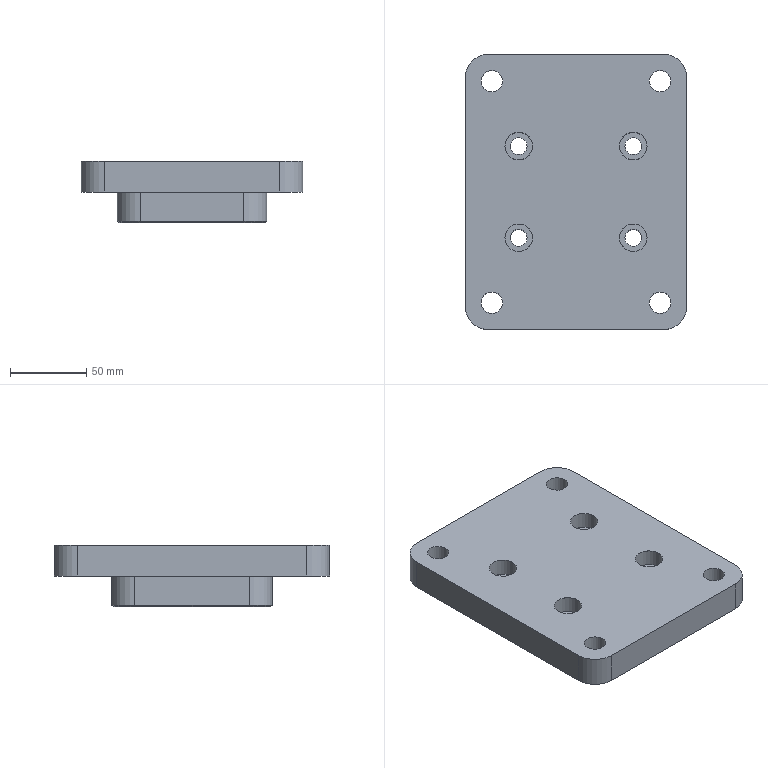NC program | NX | posted with a generic post | part box 145 x 180 x 40 mm
Lines 40 to 1301 of 5818:
(ZLEVEL_PROFILE_1_COPY , TOOL : D10)
N72 T10 M6
N74 G54
N76 G17 G0 G90 X71.61 Y79.6 S3200 M3
N78 G43 Z30. H10
N80 Z1.78
N82 G94 G1 Z-0.22 F2200.
N84 X72.478 Y78.099
N86 G3 X73.345 Y77.599 R1.
N88 G1 X74.677 Y77.6
N90 X75.
N92 G2 X95.1 Y57.5 R20.1
N94 G1 Y57.177
N96 Y55.845
N98 G3 X95.6 Y54.979 R1.
N100 G1 X97.1 Y54.112
N102 Z1.78
N104 G0 Z30.
N106 Z1.56
N108 G1 Z-0.44
N110 X95.6 Y54.979
N112 G2 X95.1 Y55.845 R1.
N114 G1 Y57.177
N116 Y57.5
N118 G3 X75. Y77.6 R20.1
N120 G1 X74.677
N122 X73.345 Y77.599
N124 G2 X72.478 Y78.099 R1.
N126 G1 X71.61 Y79.6
N128 Z1.56
N130 G0 Z30.
N132 Z1.341
N134 G1 Z-0.659
N136 X72.478 Y78.099
N138 G3 X73.345 Y77.599 R1.
N140 G1 X74.677 Y77.6
N142 X75.
N144 G2 X95.1 Y57.5 R20.1
N146 G1 Y57.177
N148 Y55.845
N150 G3 X95.6 Y54.979 R1.
N152 G1 X97.1 Y54.112
N154 Z1.341
N156 G0 Z30.
N158 Z1.121
N160 G1 Z-0.879
N162 X95.6 Y54.979
N164 G2 X95.1 Y55.845 R1.
N166 G1 Y57.177
N168 Y57.5
N170 G3 X75. Y77.6 R20.1
N172 G1 X74.677
N174 X73.345 Y77.599
N176 G2 X72.478 Y78.099 R1.
N178 G1 X71.61 Y79.6
N180 Z1.121
N182 G0 Z30.
N184 Z0.901
N186 G1 Z-1.099
N188 X72.478 Y78.099
N190 G3 X73.345 Y77.599 R1.
N192 G1 X74.677 Y77.6
N194 X75.
N196 G2 X95.1 Y57.5 R20.1
N198 G1 Y57.177
N200 Y55.845
N202 G3 X95.6 Y54.979 R1.
N204 G1 X97.1 Y54.112
N206 Z0.901
N208 G0 Z30.
N210 Z0.681
N212 G1 Z-1.319
N214 X95.6 Y54.979
N216 G2 X95.1 Y55.845 R1.
N218 G1 Y57.177
N220 Y57.5
N222 G3 X75. Y77.6 R20.1
N224 G1 X74.677
N226 X73.345 Y77.599
N228 G2 X72.478 Y78.099 R1.
N230 G1 X71.61 Y79.6
N232 Z0.681
N234 G0 Z30.
N236 Z0.462
N238 G1 Z-1.538
N240 X72.478 Y78.099
N242 G3 X73.345 Y77.599 R1.
N244 G1 X74.677 Y77.6
N246 X75.
N248 G2 X95.1 Y57.5 R20.1
N250 G1 Y57.177
N252 Y55.845
N254 G3 X95.6 Y54.979 R1.
N256 G1 X97.1 Y54.112
N258 Z0.462
N260 G0 Z30.
N262 Z0.242
N264 G1 Z-1.758
N266 X95.6 Y54.979
N268 G2 X95.1 Y55.845 R1.
N270 G1 Y57.177
N272 Y57.5
N274 G3 X75. Y77.6 R20.1
N276 G1 X74.677
N278 X73.345 Y77.599
N280 G2 X72.478 Y78.099 R1.
N282 G1 X71.61 Y79.6
N284 Z0.242
N286 G0 Z30.
N288 Z0.022
N290 G1 Z-1.978
N292 X72.478 Y78.099
N294 G3 X73.345 Y77.599 R1.
N296 G1 X74.677 Y77.6
N298 X75.
N300 G2 X95.1 Y57.5 R20.1
N302 G1 Y57.177
N304 Y55.845
N306 G3 X95.6 Y54.979 R1.
N308 G1 X97.1 Y54.112
N310 Z0.022
N312 G0 Z30.
N314 Z-0.198
N316 G1 Z-2.198
N318 X95.6 Y54.979
N320 G2 X95.1 Y55.845 R1.
N322 G1 Y57.177
N324 Y57.5
N326 G3 X75. Y77.6 R20.1
N328 G1 X74.677
N330 X73.345 Y77.599
N332 G2 X72.478 Y78.099 R1.
N334 G1 X71.61 Y79.6
N336 Z-0.198
N338 G0 Z30.
N340 Z-0.418
N342 G1 Z-2.418
N344 X72.478 Y78.099
N346 G3 X73.345 Y77.599 R1.
N348 G1 X74.677 Y77.6
N350 X75.
N352 G2 X95.1 Y57.5 R20.1
N354 G1 Y57.177
N356 Y55.845
N358 G3 X95.6 Y54.979 R1.
N360 G1 X97.1 Y54.112
N362 Z-0.418
N364 G0 Z30.
N366 Z-0.637
N368 G1 Z-2.637
N370 X95.6 Y54.979
N372 G2 X95.1 Y55.845 R1.
N374 G1 Y57.177
N376 Y57.5
N378 G3 X75. Y77.6 R20.1
N380 G1 X74.677
N382 X73.345 Y77.599
N384 G2 X72.478 Y78.099 R1.
N386 G1 X71.61 Y79.6
N388 Z-0.637
N390 G0 Z30.
N392 Z-0.857
N394 G1 Z-2.857
N396 X72.478 Y78.099
N398 G3 X73.345 Y77.599 R1.
N400 G1 X74.677 Y77.6
N402 X75.
N404 G2 X95.1 Y57.5 R20.1
N406 G1 Y57.177
N408 Y55.845
N410 G3 X95.6 Y54.979 R1.
N412 G1 X97.1 Y54.112
N414 Z-0.857
N416 G0 Z30.
N418 Z-1.077
N420 G1 Z-3.077
N422 X95.6 Y54.979
N424 G2 X95.1 Y55.845 R1.
N426 G1 Y57.177
N428 Y57.5
N430 G3 X75. Y77.6 R20.1
N432 G1 X74.677
N434 X73.345 Y77.599
N436 G2 X72.478 Y78.099 R1.
N438 G1 X71.61 Y79.6
N440 Z-1.077
N442 G0 Z30.
N444 Z-1.297
N446 G1 Z-3.297
N448 X72.478 Y78.099
N450 G3 X73.345 Y77.599 R1.
N452 G1 X74.677 Y77.6
N454 X75.
N456 G2 X95.1 Y57.5 R20.1
N458 G1 Y57.177
N460 Y55.845
N462 G3 X95.6 Y54.979 R1.
N464 G1 X97.1 Y54.112
N466 Z-1.297
N468 G0 Z30.
N470 Z-1.516
N472 G1 Z-3.516
N474 X95.6 Y54.979
N476 G2 X95.1 Y55.845 R1.
N478 G1 Y57.177
N480 Y57.5
N482 G3 X75. Y77.6 R20.1
N484 G1 X74.677
N486 X73.345 Y77.599
N488 G2 X72.478 Y78.099 R1.
N490 G1 X71.61 Y79.6
N492 Z-1.516
N494 G0 Z30.
N496 Z-1.736
N498 G1 Z-3.736
N500 X72.478 Y78.099
N502 G3 X73.345 Y77.599 R1.
N504 G1 X74.677 Y77.6
N506 X75.
N508 G2 X95.1 Y57.5 R20.1
N510 G1 Y57.177
N512 Y55.845
N514 G3 X95.6 Y54.979 R1.
N516 G1 X97.1 Y54.112
N518 Z-1.736
N520 G0 Z30.
N522 Z-1.956
N524 G1 Z-3.956
N526 X95.6 Y54.979
N528 G2 X95.1 Y55.845 R1.
N530 G1 Y57.177
N532 Y57.5
N534 G3 X75. Y77.6 R20.1
N536 G1 X74.677
N538 X73.345 Y77.599
N540 G2 X72.478 Y78.099 R1.
N542 G1 X71.61 Y79.6
N544 Z-1.956
N546 G0 Z30.
N548 Z-2.176
N550 G1 Z-4.176
N552 X72.478 Y78.099
N554 G3 X73.345 Y77.599 R1.
N556 G1 X74.677 Y77.6
N558 X75.
N560 G2 X95.1 Y57.5 R20.1
N562 G1 Y57.177
N564 Y55.845
N566 G3 X95.6 Y54.979 R1.
N568 G1 X97.1 Y54.112
N570 Z-2.176
N572 G0 Z30.
N574 Z-2.396
N576 G1 Z-4.396
N578 X95.6 Y54.979
N580 G2 X95.1 Y55.845 R1.
N582 G1 Y57.177
N584 Y57.5
N586 G3 X75. Y77.6 R20.1
N588 G1 X74.677
N590 X73.345 Y77.599
N592 G2 X72.478 Y78.099 R1.
N594 G1 X71.61 Y79.6
N596 Z-2.396
N598 G0 Z30.
N600 Z-2.615
N602 G1 Z-4.615
N604 X72.478 Y78.099
N606 G3 X73.345 Y77.599 R1.
N608 G1 X74.677 Y77.6
N610 X75.
N612 G2 X95.1 Y57.5 R20.1
N614 G1 Y57.177
N616 Y55.845
N618 G3 X95.6 Y54.979 R1.
N620 G1 X97.1 Y54.112
N622 Z-2.615
N624 G0 Z30.
N626 Z-2.835
N628 G1 Z-4.835
N630 X95.6 Y54.979
N632 G2 X95.1 Y55.845 R1.
N634 G1 Y57.177
N636 Y57.5
N638 G3 X75. Y77.6 R20.1
N640 G1 X74.677
N642 X73.345 Y77.599
N644 G2 X72.478 Y78.099 R1.
N646 G1 X71.61 Y79.6
N648 Z-2.835
N650 G0 Z30.
N652 Z-3.055
N654 G1 Z-5.055
N656 X72.478 Y78.099
N658 G3 X73.345 Y77.599 R1.
N660 G1 X74.677 Y77.6
N662 X75.
N664 G2 X95.1 Y57.5 R20.1
N666 G1 Y57.177
N668 Y55.845
N670 G3 X95.6 Y54.979 R1.
N672 G1 X97.1 Y54.112
N674 Z-3.055
N676 G0 Z30.
N678 Z-3.275
N680 G1 Z-5.275
N682 X95.6 Y54.979
N684 G2 X95.1 Y55.845 R1.
N686 G1 Y57.177
N688 Y57.5
N690 G3 X75. Y77.6 R20.1
N692 G1 X74.677
N694 X73.345 Y77.599
N696 G2 X72.478 Y78.099 R1.
N698 G1 X71.61 Y79.6
N700 Z-3.275
N702 G0 Z30.
N704 Z-3.495
N706 G1 Z-5.495
N708 X72.478 Y78.099
N710 G3 X73.345 Y77.599 R1.
N712 G1 X74.677 Y77.6
N714 X75.
N716 G2 X95.1 Y57.5 R20.1
N718 G1 Y57.177
N720 Y55.845
N722 G3 X95.6 Y54.979 R1.
N724 G1 X97.1 Y54.112
N726 Z-3.495
N728 G0 Z30.
N730 Z-3.714
N732 G1 Z-5.714
N734 X95.6 Y54.979
N736 G2 X95.1 Y55.845 R1.
N738 G1 Y57.177
N740 Y57.5
N742 G3 X75. Y77.6 R20.1
N744 G1 X74.677
N746 X73.345 Y77.599
N748 G2 X72.478 Y78.099 R1.
N750 G1 X71.61 Y79.6
N752 Z-3.714
N754 G0 Z30.
N756 Z-3.934
N758 G1 Z-5.934
N760 X72.478 Y78.099
N762 G3 X73.345 Y77.599 R1.
N764 G1 X74.677 Y77.6
N766 X75.
N768 G2 X95.1 Y57.5 R20.1
N770 G1 Y57.177
N772 Y55.845
N774 G3 X95.6 Y54.979 R1.
N776 G1 X97.1 Y54.112
N778 Z-3.934
N780 G0 Z30.
N782 Z-4.154
N784 G1 Z-6.154
N786 X95.6 Y54.979
N788 G2 X95.1 Y55.845 R1.
N790 G1 Y57.177
N792 Y57.5
N794 G3 X75. Y77.6 R20.1
N796 G1 X74.677
N798 X73.345 Y77.599
N800 G2 X72.478 Y78.099 R1.
N802 G1 X71.61 Y79.6
N804 Z-4.154
N806 G0 Z30.
N808 Z-4.374
N810 G1 Z-6.374
N812 X72.478 Y78.099
N814 G3 X73.345 Y77.599 R1.
N816 G1 X74.677 Y77.6
N818 X75.
N820 G2 X95.1 Y57.5 R20.1
N822 G1 Y57.177
N824 Y55.845
N826 G3 X95.6 Y54.979 R1.
N828 G1 X97.1 Y54.112
N830 Z-4.374
N832 G0 Z30.
N834 Z-4.593
N836 G1 Z-6.593
N838 X95.6 Y54.979
N840 G2 X95.1 Y55.845 R1.
N842 G1 Y57.177
N844 Y57.5
N846 G3 X75. Y77.6 R20.1
N848 G1 X74.677
N850 X73.345 Y77.599
N852 G2 X72.478 Y78.099 R1.
N854 G1 X71.61 Y79.6
N856 Z-4.593
N858 G0 Z30.
N860 Z-4.813
N862 G1 Z-6.813
N864 X72.478 Y78.099
N866 G3 X73.345 Y77.599 R1.
N868 G1 X74.677 Y77.6
N870 X75.
N872 G2 X95.1 Y57.5 R20.1
N874 G1 Y57.177
N876 Y55.845
N878 G3 X95.6 Y54.979 R1.
N880 G1 X97.1 Y54.112
N882 Z-4.813
N884 G0 Z30.
N886 Z-5.033
N888 G1 Z-7.033
N890 X95.6 Y54.979
N892 G2 X95.1 Y55.845 R1.
N894 G1 Y57.177
N896 Y57.5
N898 G3 X75. Y77.6 R20.1
N900 G1 X74.677
N902 X73.345 Y77.599
N904 G2 X72.478 Y78.099 R1.
N906 G1 X71.61 Y79.6
N908 Z-5.033
N910 G0 Z30.
N912 Z-5.253
N914 G1 Z-7.253
N916 X72.478 Y78.099
N918 G3 X73.345 Y77.599 R1.
N920 G1 X74.677 Y77.6
N922 X75.
N924 G2 X95.1 Y57.5 R20.1
N926 G1 Y57.177
N928 Y55.845
N930 G3 X95.6 Y54.979 R1.
N932 G1 X97.1 Y54.112
N934 Z-5.253
N936 G0 Z30.
N938 Z-5.473
N940 G1 Z-7.473
N942 X95.6 Y54.979
N944 G2 X95.1 Y55.845 R1.
N946 G1 Y57.177
N948 Y57.5
N950 G3 X75. Y77.6 R20.1
N952 G1 X74.677
N954 X73.345 Y77.599
N956 G2 X72.478 Y78.099 R1.
N958 G1 X71.61 Y79.6
N960 Z-5.473
N962 G0 Z30.
N964 Z-5.692
N966 G1 Z-7.692
N968 X72.478 Y78.099
N970 G3 X73.345 Y77.599 R1.
N972 G1 X74.677 Y77.6
N974 X75.
N976 G2 X95.1 Y57.5 R20.1
N978 G1 Y57.177
N980 Y55.845
N982 G3 X95.6 Y54.979 R1.
N984 G1 X97.1 Y54.112
N986 Z-5.692
N988 G0 Z30.
N990 Z-5.912
N992 G1 Z-7.912
N994 X95.6 Y54.979
N996 G2 X95.1 Y55.845 R1.
N998 G1 Y57.177
N1000 Y57.5
N1002 G3 X75. Y77.6 R20.1
N1004 G1 X74.677
N1006 X73.345 Y77.599
N1008 G2 X72.478 Y78.099 R1.
N1010 G1 X71.61 Y79.6
N1012 Z-5.912
N1014 G0 Z30.
N1016 Z-6.132
N1018 G1 Z-8.132
N1020 X72.478 Y78.099
N1022 G3 X73.345 Y77.599 R1.
N1024 G1 X74.677 Y77.6
N1026 X75.
N1028 G2 X95.1 Y57.5 R20.1
N1030 G1 Y57.177
N1032 Y55.845
N1034 G3 X95.6 Y54.979 R1.
N1036 G1 X97.1 Y54.112
N1038 Z-6.132
N1040 G0 Z30.
N1042 Z-6.352
N1044 G1 Z-8.352
N1046 X95.6 Y54.979
N1048 G2 X95.1 Y55.845 R1.
N1050 G1 Y57.177
N1052 Y57.5
N1054 G3 X75. Y77.6 R20.1
N1056 G1 X74.677
N1058 X73.345 Y77.599
N1060 G2 X72.478 Y78.099 R1.
N1062 G1 X71.61 Y79.6
N1064 Z-6.352
N1066 G0 Z30.
N1068 Z-6.571
N1070 G1 Z-8.571
N1072 X72.478 Y78.099
N1074 G3 X73.345 Y77.599 R1.
N1076 G1 X74.677 Y77.6
N1078 X75.
N1080 G2 X95.1 Y57.5 R20.1
N1082 G1 Y57.177
N1084 Y55.845
N1086 G3 X95.6 Y54.979 R1.
N1088 G1 X97.1 Y54.112
N1090 Z-6.571
N1092 G0 Z30.
N1094 Z-6.791
N1096 G1 Z-8.791
N1098 X95.6 Y54.979
N1100 G2 X95.1 Y55.845 R1.
N1102 G1 Y57.177
N1104 Y57.5
N1106 G3 X75. Y77.6 R20.1
N1108 G1 X74.677
N1110 X73.345 Y77.599
N1112 G2 X72.478 Y78.099 R1.
N1114 G1 X71.61 Y79.6
N1116 Z-6.791
N1118 G0 Z30.
N1120 Z-7.011
N1122 G1 Z-9.011
N1124 X72.478 Y78.099
N1126 G3 X73.345 Y77.599 R1.
N1128 G1 X74.677 Y77.6
N1130 X75.
N1132 G2 X95.1 Y57.5 R20.1
N1134 G1 Y57.177
N1136 Y55.845
N1138 G3 X95.6 Y54.979 R1.
N1140 G1 X97.1 Y54.112
N1142 Z-7.011
N1144 G0 Z30.
N1146 Z-7.231
N1148 G1 Z-9.231
N1150 X95.6 Y54.979
N1152 G2 X95.1 Y55.845 R1.
N1154 G1 Y57.177
N1156 Y57.5
N1158 G3 X75. Y77.6 R20.1
N1160 G1 X74.677
N1162 X73.345 Y77.599
N1164 G2 X72.478 Y78.099 R1.
N1166 G1 X71.61 Y79.6
N1168 Z-7.231
N1170 G0 Z30.
N1172 Z-7.451
N1174 G1 Z-9.451
N1176 X72.478 Y78.099
N1178 G3 X73.345 Y77.599 R1.
N1180 G1 X74.677 Y77.6
N1182 X75.
N1184 G2 X95.1 Y57.5 R20.1
N1186 G1 Y57.177
N1188 Y55.845
N1190 G3 X95.6 Y54.979 R1.
N1192 G1 X97.1 Y54.112
N1194 Z-7.451
N1196 G0 Z30.
N1198 Z-7.67
N1200 G1 Z-9.67
N1202 X95.6 Y54.979
N1204 G2 X95.1 Y55.845 R1.
N1206 G1 Y57.177
N1208 Y57.5
N1210 G3 X75. Y77.6 R20.1
N1212 G1 X74.677
N1214 X73.345 Y77.599
N1216 G2 X72.478 Y78.099 R1.
N1218 G1 X71.61 Y79.6
N1220 Z-7.67
N1222 G0 Z30.
N1224 Z-7.89
N1226 G1 Z-9.89
N1228 X72.478 Y78.099
N1230 G3 X73.345 Y77.599 R1.
N1232 G1 X74.677 Y77.6
N1234 X75.
N1236 G2 X95.1 Y57.5 R20.1
N1238 G1 Y57.177
N1240 Y55.845
N1242 G3 X95.6 Y54.979 R1.
N1244 G1 X97.1 Y54.112
N1246 Z-7.89
N1248 G0 Z30.
N1250 Z-8.11
N1252 G1 Z-10.11
N1254 X95.6 Y54.979
N1256 G2 X95.1 Y55.845 R1.
N1258 G1 Y57.177
N1260 Y57.5
N1262 G3 X75. Y77.6 R20.1
N1264 G1 X74.677
N1266 X73.345 Y77.599
N1268 G2 X72.478 Y78.099 R1.
N1270 G1 X71.61 Y79.6
N1272 Z-8.11
N1274 G0 Z30.
N1276 X71.611 Z-8.33
N1278 G1 Z-10.33
N1280 X72.478 Y78.099
N1282 G3 X73.345 Y77.599 R1.
N1284 G1 X74.677 Y77.6
N1286 X75.
N1288 G2 X95.1 Y57.5 R20.1
N1290 G1 Y57.177
N1292 Y55.845
N1294 G3 X95.6 Y54.979 R1.
N1296 G1 X97.1 Y54.112
N1298 Z-8.33
N1300 G0 Z30.
N1302 Z-8.549
N1304 G1 Z-10.549
N1306 X95.6 Y54.979
N1308 G2 X95.1 Y55.845 R1.
N1310 G1 Y57.177
N1312 Y57.5
N1314 G3 X75. Y77.6 R20.1
N1316 G1 X74.677
N1318 X73.345 Y77.599
N1320 G2 X72.478 Y78.099 R1.
N1322 G1 X71.611 Y79.6
N1324 Z-8.549
N1326 G0 Z30.
N1328 Z-8.769
N1330 G1 Z-10.769
N1332 X72.478 Y78.099
N1334 G3 X73.345 Y77.599 R1.
N1336 G1 X74.677 Y77.6
N1338 X75.
N1340 G2 X95.1 Y57.5 R20.1
N1342 G1 Y57.177
N1344 Y55.845
N1346 G3 X95.6 Y54.979 R1.
N1348 G1 X97.1 Y54.112
N1350 Z-8.769
N1352 G0 Z30.
N1354 Z-8.989
N1356 G1 Z-10.989
N1358 X95.6 Y54.979
N1360 G2 X95.1 Y55.845 R1.
N1362 G1 Y57.177
N1364 Y57.5
N1366 G3 X75. Y77.6 R20.1
N1368 G1 X74.677
N1370 X73.345 Y77.599
N1372 G2 X72.478 Y78.099 R1.
N1374 G1 X71.611 Y79.6
N1376 Z-8.989
N1378 G0 Z30.
N1380 Z-9.209
N1382 G1 Z-11.209
N1384 X72.478 Y78.099
N1386 G3 X73.345 Y77.599 R1.
N1388 G1 X74.677 Y77.6
N1390 X75.
N1392 G2 X95.1 Y57.5 R20.1
N1394 G1 Y57.177
N1396 Y55.845
N1398 G3 X95.6 Y54.979 R1.
N1400 G1 X97.1 Y54.112
N1402 Z-9.209
N1404 G0 Z30.
N1406 Z-9.429
N1408 G1 Z-11.429
N1410 X95.6 Y54.979
N1412 G2 X95.1 Y55.845 R1.
N1414 G1 Y57.177
N1416 Y57.5
N1418 G3 X75. Y77.6 R20.1
N1420 G1 X74.677
N1422 X73.345 Y77.599
N1424 G2 X72.478 Y78.099 R1.
N1426 G1 X71.611 Y79.6
N1428 Z-9.429
N1430 G0 Z30.
N1432 Z-9.648
N1434 G1 Z-11.648
N1436 X72.478 Y78.099
N1438 G3 X73.345 Y77.599 R1.
N1440 G1 X74.677 Y77.6
N1442 X75.
N1444 G2 X95.1 Y57.5 R20.1
N1446 G1 Y57.177
N1448 Y55.845
N1450 G3 X95.6 Y54.979 R1.
N1452 G1 X97.1 Y54.112
N1454 Z-9.648
N1456 G0 Z30.
N1458 Z-9.868
N1460 G1 Z-11.868
N1462 X95.6 Y54.979
N1464 G2 X95.1 Y55.845 R1.
N1466 G1 Y57.177
N1468 Y57.5
N1470 G3 X75. Y77.6 R20.1
N1472 G1 X74.677
N1474 X73.345 Y77.599
N1476 G2 X72.478 Y78.099 R1.
N1478 G1 X71.611 Y79.6
N1480 Z-9.868
N1482 G0 Z30.
N1484 Z-10.088
N1486 G1 Z-12.088
N1488 X72.478 Y78.099
N1490 G3 X73.345 Y77.599 R1.
N1492 G1 X74.677 Y77.6
N1494 X75.
N1496 G2 X95.1 Y57.5 R20.1
N1498 G1 Y57.177
N1500 Y55.845
N1502 G3 X95.6 Y54.979 R1.
N1504 G1 X97.1 Y54.112
N1506 Z-10.088
N1508 G0 Z30.
N1510 Z-10.308
N1512 G1 Z-12.308
N1514 X95.6 Y54.979
N1516 G2 X95.1 Y55.845 R1.
N1518 G1 Y57.177
N1520 Y57.5
N1522 G3 X75. Y77.6 R20.1
N1524 G1 X74.677
N1526 X73.345 Y77.599
N1528 G2 X72.478 Y78.099 R1.
N1530 G1 X71.611 Y79.6
N1532 Z-10.308
N1534 G0 Z30.
N1536 Z-10.527
N1538 G1 Z-12.527
N1540 X72.478 Y78.099
N1542 G3 X73.345 Y77.599 R1.
N1544 G1 X74.677 Y77.6
N1546 X75.
N1548 G2 X95.1 Y57.5 R20.1
N1550 G1 Y57.177
N1552 Y55.845
N1554 G3 X95.6 Y54.979 R1.
N1556 G1 X97.1 Y54.112
N1558 Z-10.527
N1560 G0 Z30.
N1562 Z-10.747
N1564 G1 Z-12.747
N1566 X95.6 Y54.979
N1568 G2 X95.1 Y55.845 R1.
N1570 G1 Y57.177
N1572 Y57.5
N1574 G3 X75. Y77.6 R20.1
N1576 G1 X74.677
N1578 X73.345 Y77.599
N1580 G2 X72.478 Y78.099 R1.
N1582 G1 X71.611 Y79.6
N1584 Z-10.747
N1586 G0 Z30.
N1588 Z-10.967
N1590 G1 Z-12.967
N1592 X72.478 Y78.099
N1594 G3 X73.345 Y77.599 R1.
N1596 G1 X74.677 Y77.6
N1598 X75.
N1600 G2 X95.1 Y57.5 R20.1
N1602 G1 Y57.177
N1604 Y55.845
N1606 G3 X95.6 Y54.979 R1.
N1608 G1 X97.1 Y54.112
N1610 Z-10.967
N1612 G0 Z30.
N1614 Z-11.187
N1616 G1 Z-13.187
N1618 X95.6 Y54.979
N1620 G2 X95.1 Y55.845 R1.
N1622 G1 Y57.177
N1624 Y57.5
N1626 G3 X75. Y77.6 R20.1
N1628 G1 X74.677
N1630 X73.345 Y77.599
N1632 G2 X72.478 Y78.099 R1.
N1634 G1 X71.611 Y79.6
N1636 Z-11.187
N1638 G0 Z30.
N1640 Z-11.407
N1642 G1 Z-13.407
N1644 X72.478 Y78.099
N1646 G3 X73.345 Y77.599 R1.
N1648 G1 X74.677 Y77.6
N1650 X75.
N1652 G2 X95.1 Y57.5 R20.1
N1654 G1 Y57.177
N1656 Y55.845
N1658 G3 X95.6 Y54.979 R1.
N1660 G1 X97.1 Y54.112
N1662 Z-11.407
N1664 G0 Z30.
N1666 Z-11.626
N1668 G1 Z-13.626
N1670 X95.6 Y54.979
N1672 G2 X95.1 Y55.845 R1.
N1674 G1 Y57.177
N1676 Y57.5
N1678 G3 X75. Y77.6 R20.1
N1680 G1 X74.677
N1682 X73.345 Y77.599
N1684 G2 X72.478 Y78.099 R1.
N1686 G1 X71.611 Y79.6
N1688 Z-11.626
N1690 G0 Z30.
N1692 Z-11.846
N1694 G1 Z-13.846
N1696 X72.478 Y78.099
N1698 G3 X73.345 Y77.599 R1.
N1700 G1 X74.677 Y77.6
N1702 X75.
N1704 G2 X95.1 Y57.5 R20.1
N1706 G1 Y57.177
N1708 Y55.845
N1710 G3 X95.6 Y54.979 R1.
N1712 G1 X97.1 Y54.112
N1714 Z-11.846
N1716 G0 Z30.
N1718 Z-12.066
N1720 G1 Z-14.066
N1722 X95.6 Y54.979
N1724 G2 X95.1 Y55.845 R1.
N1726 G1 Y57.177
N1728 Y57.5
N1730 G3 X75. Y77.6 R20.1
N1732 G1 X74.677
N1734 X73.345 Y77.599
N1736 G2 X72.478 Y78.099 R1.
N1738 G1 X71.611 Y79.6
N1740 Z-12.066
N1742 G0 Z30.
N1744 Z-12.286
N1746 G1 Z-14.286
N1748 X72.478 Y78.099
N1750 G3 X73.345 Y77.599 R1.
N1752 G1 X74.677 Y77.6
N1754 X75.
N1756 G2 X95.1 Y57.5 R20.1
N1758 G1 Y57.177
N1760 Y55.845
N1762 G3 X95.6 Y54.979 R1.
N1764 G1 X97.1 Y54.112
N1766 Z-12.286
N1768 G0 Z30.
N1770 Z-12.505
N1772 G1 Z-14.505
N1774 X95.6 Y54.979
N1776 G2 X95.1 Y55.845 R1.
N1778 G1 Y57.177
N1780 Y57.5
N1782 G3 X75. Y77.6 R20.1
N1784 G1 X74.677
N1786 X73.345 Y77.599
N1788 G2 X72.478 Y78.099 R1.
N1790 G1 X71.611 Y79.6
N1792 Z-12.505
N1794 G0 Z30.
N1796 Z-12.725
N1798 G1 Z-14.725
N1800 X72.478 Y78.099
N1802 G3 X73.345 Y77.599 R1.
N1804 G1 X74.677 Y77.6
N1806 X75.
N1808 G2 X95.1 Y57.5 R20.1
N1810 G1 Y57.177
N1812 Y55.845
N1814 G3 X95.6 Y54.979 R1.
N1816 G1 X97.1 Y54.112
N1818 Z-12.725
N1820 G0 Z30.
N1822 Y54.113 Z-12.945
N1824 G1 Z-14.945
N1826 X95.6 Y54.979
N1828 G2 X95.1 Y55.845 R1.
N1830 G1 Y57.177
N1832 Y57.5
N1834 G3 X75. Y77.6 R20.1
N1836 G1 X74.677
N1838 X73.345 Y77.599
N1840 G2 X72.478 Y78.099 R1.
N1842 G1 X71.611 Y79.6
N1844 Z-12.945
N1846 G0 Z30.
N1848 Z-13.165
N1850 G1 Z-15.165
N1852 X72.478 Y78.099
N1854 G3 X73.345 Y77.599 R1.
N1856 G1 X74.677 Y77.6
N1858 X75.
N1860 G2 X95.1 Y57.5 R20.1
N1862 G1 Y57.177
N1864 Y55.845
N1866 G3 X95.6 Y54.979 R1.
N1868 G1 X97.1 Y54.113
N1870 Z-13.165
N1872 G0 Z30.
N1874 Z-13.385
N1876 G1 Z-15.385
N1878 X95.6 Y54.979
N1880 G2 X95.1 Y55.845 R1.
N1882 G1 Y57.177
N1884 Y57.5
N1886 G3 X75. Y77.6 R20.1
N1888 G1 X74.677
N1890 X73.345 Y77.599
N1892 G2 X72.478 Y78.099 R1.
N1894 G1 X71.611 Y79.6
N1896 Z-13.385
N1898 G0 Z30.
N1900 Z-13.604
N1902 G1 Z-15.604
N1904 X72.478 Y78.099
N1906 G3 X73.345 Y77.599 R1.
N1908 G1 X74.677 Y77.6
N1910 X75.
N1912 G2 X95.1 Y57.5 R20.1
N1914 G1 Y57.177
N1916 Y55.845
N1918 G3 X95.6 Y54.979 R1.
N1920 G1 X97.1 Y54.113
N1922 Z-13.604
N1924 G0 Z30.
N1926 Z-13.824
N1928 G1 Z-15.824
N1930 X95.6 Y54.979
N1932 G2 X95.1 Y55.845 R1.
N1934 G1 Y57.177
N1936 Y57.5
N1938 G3 X75. Y77.6 R20.1
N1940 G1 X74.677
N1942 X73.345 Y77.599
N1944 G2 X72.478 Y78.099 R1.
N1946 G1 X71.611 Y79.6
N1948 Z-13.824
N1950 G0 Z30.
N1952 Z-14.044
N1954 G1 Z-16.044
N1956 X72.478 Y78.099
N1958 G3 X73.345 Y77.599 R1.
N1960 G1 X74.677 Y77.6
N1962 X75.
N1964 G2 X95.1 Y57.5 R20.1
N1966 G1 Y57.177
N1968 Y55.845
N1970 G3 X95.6 Y54.979 R1.
N1972 G1 X97.1 Y54.113
N1974 Z-14.044
N1976 G0 Z30.
N1978 Z-14.264
N1980 G1 Z-16.264
N1982 X95.6 Y54.979
N1984 G2 X95.1 Y55.845 R1.
N1986 G1 Y57.177
N1988 Y57.5
N1990 G3 X75. Y77.6 R20.1
N1992 G1 X74.677
N1994 X73.345 Y77.599
N1996 G2 X72.478 Y78.099 R1.
N1998 G1 X71.611 Y79.6
N2000 Z-14.264
N2002 G0 Z30.
N2004 Z-14.484
N2006 G1 Z-16.484
N2008 X72.478 Y78.099
N2010 G3 X73.345 Y77.599 R1.
N2012 G1 X74.677 Y77.6
N2014 X75.
N2016 G2 X95.1 Y57.5 R20.1
N2018 G1 Y57.177
N2020 Y55.845
N2022 G3 X95.6 Y54.979 R1.
N2024 G1 X97.1 Y54.113
N2026 Z-14.484
N2028 G0 Z30.
N2030 Z-14.703
N2032 G1 Z-16.703
N2034 X95.6 Y54.979
N2036 G2 X95.1 Y55.845 R1.
N2038 G1 Y57.177
N2040 Y57.5
N2042 G3 X75. Y77.6 R20.1
N2044 G1 X74.677
N2046 X73.345 Y77.599
N2048 G2 X72.478 Y78.099 R1.
N2050 G1 X71.611 Y79.6
N2052 Z-14.703
N2054 G0 Z30.
N2056 Z-14.923
N2058 G1 Z-16.923
N2060 X72.478 Y78.099
N2062 G3 X73.345 Y77.599 R1.
N2064 G1 X74.677 Y77.6
N2066 X75.
N2068 G2 X95.1 Y57.5 R20.1
N2070 G1 Y57.177
N2072 Y55.845
N2074 G3 X95.6 Y54.979 R1.
N2076 G1 X97.1 Y54.113
N2078 Z-14.923
N2080 G0 Z30.
N2082 Z-15.143
N2084 G1 Z-17.143
N2086 X95.6 Y54.979
N2088 G2 X95.1 Y55.845 R1.
N2090 G1 Y57.177
N2092 Y57.5
N2094 G3 X75. Y77.6 R20.1
N2096 G1 X74.677
N2098 X73.345 Y77.599
N2100 G2 X72.478 Y78.099 R1.
N2102 G1 X71.611 Y79.6
N2104 Z-15.143
N2106 G0 Z30.
N2108 Z-15.363
N2110 G1 Z-17.363
N2112 X72.478 Y78.099
N2114 G3 X73.345 Y77.599 R1.
N2116 G1 X74.677 Y77.6
N2118 X75.
N2120 G2 X95.1 Y57.5 R20.1
N2122 G1 Y57.177
N2124 Y55.845
N2126 G3 X95.6 Y54.979 R1.
N2128 G1 X97.1 Y54.113
N2130 Z-15.363
N2132 G0 Z30.
N2134 Z-15.582
N2136 G1 Z-17.582
N2138 X95.6 Y54.979
N2140 G2 X95.1 Y55.845 R1.
N2142 G1 Y57.177
N2144 Y57.5
N2146 G3 X75. Y77.6 R20.1
N2148 G1 X74.677
N2150 X73.345 Y77.599
N2152 G2 X72.478 Y78.099 R1.
N2154 G1 X71.611 Y79.6
N2156 Z-15.582
N2158 G0 Z30.
N2160 Z-15.802
N2162 G1 Z-17.802
N2164 X72.478 Y78.099
N2166 G3 X73.345 Y77.599 R1.
N2168 G1 X74.677 Y77.6
N2170 X75.
N2172 G2 X95.1 Y57.5 R20.1
N2174 G1 Y57.177
N2176 Y55.845
N2178 G3 X95.6 Y54.979 R1.
N2180 G1 X97.1 Y54.113
N2182 Z-15.802
N2184 G0 Z30.
N2186 Z-16.022
N2188 G1 Z-18.022
N2190 X95.6 Y54.979
N2192 G2 X95.1 Y55.845 R1.
N2194 G1 Y57.177
N2196 Y57.5
N2198 G3 X75. Y77.6 R20.1
N2200 G1 X74.677
N2202 X73.345 Y77.599
N2204 G2 X72.478 Y78.099 R1.
N2206 G1 X71.611 Y79.6
N2208 Z-16.022
N2210 G0 Z30.
N2212 Z-16.242
N2214 G1 Z-18.242
N2216 X72.478 Y78.099
N2218 G3 X73.345 Y77.599 R1.
N2220 G1 X74.677 Y77.6
N2222 X75.
N2224 G2 X95.1 Y57.5 R20.1
N2226 G1 Y57.177
N2228 Y55.845
N2230 G3 X95.6 Y54.979 R1.
N2232 G1 X97.1 Y54.113
N2234 Z-16.242
N2236 G0 Z30.
N2238 Z-16.462
N2240 G1 Z-18.462
N2242 X95.6 Y54.979
N2244 G2 X95.1 Y55.845 R1.
N2246 G1 Y57.177
N2248 Y57.5
N2250 G3 X75. Y77.6 R20.1
N2252 G1 X74.677
N2254 X73.345 Y77.599
N2256 G2 X72.478 Y78.099 R1.
N2258 G1 X71.611 Y79.6
N2260 Z-16.462
N2262 G0 Z30.
N2264 Z-16.681
N2266 G1 Z-18.681
N2268 X72.478 Y78.099
N2270 G3 X73.345 Y77.599 R1.
N2272 G1 X74.677 Y77.6
N2274 X75.
N2276 G2 X95.1 Y57.5 R20.1
N2278 G1 Y57.177
N2280 Y55.845
N2282 G3 X95.6 Y54.979 R1.
N2284 G1 X97.1 Y54.113
N2286 Z-16.681
N2288 G0 Z30.
N2290 Z-16.901
N2292 G1 Z-18.901
N2294 X95.6 Y54.979
N2296 G2 X95.1 Y55.845 R1.
N2298 G1 Y57.177
N2300 Y57.5
N2302 G3 X75. Y77.6 R20.1
N2304 G1 X74.677
N2306 X73.345 Y77.599
N2308 G2 X72.478 Y78.099 R1.
N2310 G1 X71.611 Y79.6
N2312 Z-16.901
N2314 G0 Z30.
N2316 Z-17.121
N2318 G1 Z-19.121
N2320 X72.478 Y78.099
N2322 G3 X73.345 Y77.599 R1.
N2324 G1 X74.677 Y77.6
N2326 X75.
N2328 G2 X95.1 Y57.5 R20.1
N2330 G1 Y57.177
N2332 Y55.845
N2334 G3 X95.6 Y54.979 R1.
N2336 G1 X97.1 Y54.113
N2338 Z-17.121
N2340 G0 Z30.
N2342 Z-17.341
N2344 G1 Z-19.341
N2346 X95.6 Y54.979
N2348 G2 X95.1 Y55.845 R1.
N2350 G1 Y57.177
N2352 Y57.5
N2354 G3 X75. Y77.6 R20.1
N2356 G1 X74.677
N2358 X73.345 Y77.599
N2360 G2 X72.478 Y78.099 R1.
N2362 G1 X71.611 Y79.6
N2364 Z-17.341
N2366 G0 Z30.
N2368 Z-17.56
N2370 G1 Z-19.56
N2372 X72.478 Y78.099
N2374 G3 X73.345 Y77.599 R1.
N2376 G1 X74.677 Y77.6
N2378 X75.
N2380 G2 X95.1 Y57.5 R20.1
N2382 G1 Y57.177
N2384 Y55.845
N2386 G3 X95.6 Y54.979 R1.
N2388 G1 X97.1 Y54.113
N2390 Z-17.56
N2392 G0 Z30.
N2394 Z-17.78
N2396 G1 Z-19.78
N2398 X95.6 Y54.979
N2400 G2 X95.1 Y55.845 R1.
N2402 G1 Y57.177
N2404 Y57.5
N2406 G3 X75. Y77.6 R20.1
N2408 G1 X74.677
N2410 X73.345 Y77.599
N2412 G2 X72.478 Y78.099 R1.
N2414 G1 X71.611 Y79.6
N2416 Z-17.78
N2418 G0 Z30.
N2420 Z-18.
N2422 G1 Z-20.
N2424 X72.478 Y78.099
N2426 G3 X73.345 Y77.599 R1.
N2428 G1 X74.677 Y77.6
N2430 X75.
N2432 G2 X95.1 Y57.5 R20.1
N2434 G1 Y57.177
N2436 Y55.845
N2438 G3 X95.6 Y54.979 R1.
N2440 G1 X97.1 Y54.113
N2442 Z-18.
N2444 G0 Z30.
N2446 Y-54.112
N2448 Z1.78
N2450 G1 Z-0.22
N2452 X95.6 Y-54.979
N2454 G3 X95.1 Y-55.845 R1.
N2456 G1 Y-57.177
N2458 Y-57.5
N2460 G2 X75. Y-77.6 R20.1
N2462 G1 X74.677
N2464 X73.345
N2466 G3 X72.479 Y-78.1 R1.
N2468 G1 X71.612 Y-79.6
N2470 Z1.78
N2472 G0 Z30.
N2474 Z1.56
N2476 G1 Z-0.44
N2478 X72.479 Y-78.1
N2480 G2 X73.345 Y-77.6 R1.
N2482 G1 X74.677
N2484 X75.
N2486 G3 X95.1 Y-57.5 R20.1
N2488 G1 Y-57.177
N2490 Y-55.845
N2492 G2 X95.6 Y-54.979 R1.
N2494 G1 X97.1 Y-54.112
N2496 Z1.56
N2498 G0 Z30.
N2500 Z1.341
N2502 G1 Z-0.659
N2504 X95.6 Y-54.979
N2506 G3 X95.1 Y-55.845 R1.
N2508 G1 Y-57.177
N2510 Y-57.5
N2512 G2 X75. Y-77.6 R20.1
N2514 G1 X74.677
N2516 X73.345
N2518 G3 X72.479 Y-78.1 R1.
N2520 G1 X71.612 Y-79.6
N2522 Z1.341
N2524 G0 Z30.
N2526 Z1.121
N2528 G1 Z-0.879
N2530 X72.479 Y-78.1
N2532 G2 X73.345 Y-77.6 R1.
N2534 G1 X74.677
N2536 X75.
N2538 G3 X95.1 Y-57.5 R20.1
N2540 G1 Y-57.177
N2542 Y-55.845
N2544 G2 X95.6 Y-54.979 R1.
N2546 G1 X97.1 Y-54.112
N2548 Z1.121
N2550 G0 Z30.
N2552 Z0.901
N2554 G1 Z-1.099
N2556 X95.6 Y-54.979
N2558 G3 X95.1 Y-55.845 R1.
N2560 G1 Y-57.177
N2562 Y-57.5
N2564 G2 X75. Y-77.6 R20.1
N2566 G1 X74.677
N2568 X73.345
N2570 G3 X72.479 Y-78.1 R1.
N2572 G1 X71.612 Y-79.6
N2574 Z0.901
N2576 G0 Z30.
N2578 Z0.681
N2580 G1 Z-1.319
N2582 X72.479 Y-78.1
N2584 G2 X73.345 Y-77.6 R1.
N2586 G1 X74.677
N2588 X75.